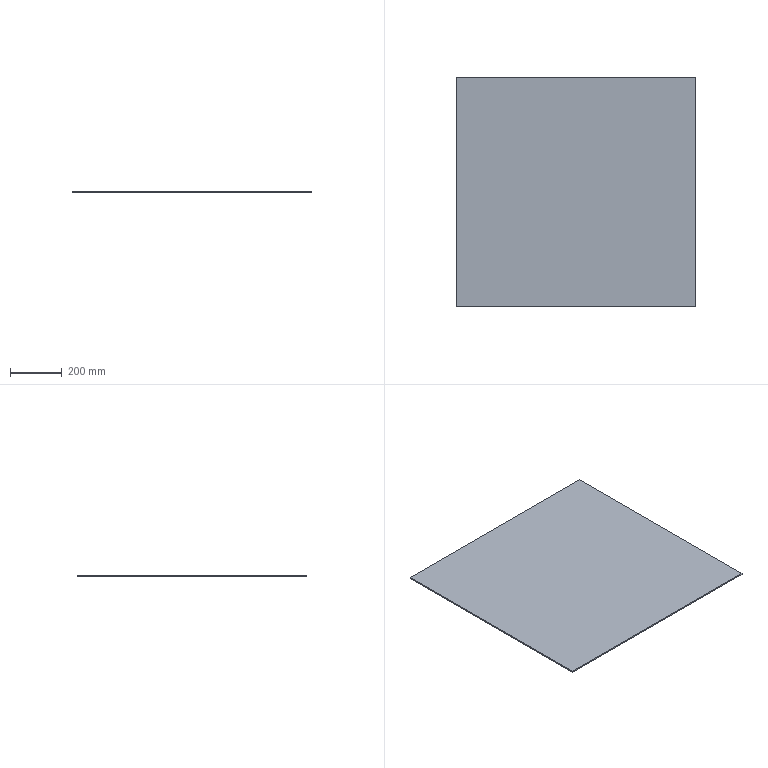Part | SolidWorks | features Extrusion 1 | 1 solid | 6 faces | box 926 x 887 x 5 mm | volume 4106810 mm3 | plane 6
STEP:
#1=CARTESIAN_POINT('',(463.,-443.5,0.));
#2=VERTEX_POINT('',#1);
#3=CARTESIAN_POINT('',(463.,443.5,0.));
#4=VERTEX_POINT('',#3);
#5=CARTESIAN_POINT('',(463.,443.5,0.));
#6=DIRECTION('',(0.,1.,0.));
#7=VECTOR('',#6,1000.);
#8=LINE('',#5,#7);
#9=EDGE_CURVE('',#2,#4,#8,.T.);
#10=ORIENTED_EDGE('',*,*,#9,.T.);
#11=CARTESIAN_POINT('',(463.,443.5,5.));
#12=VERTEX_POINT('',#11);
#13=CARTESIAN_POINT('',(463.,443.5,5.));
#14=DIRECTION('',(0.,0.,-1.));
#15=VECTOR('',#14,1000.);
#16=LINE('',#13,#15);
#17=EDGE_CURVE('',#12,#4,#16,.T.);
#18=ORIENTED_EDGE('',*,*,#17,.F.);
#19=CARTESIAN_POINT('',(463.,-443.5,5.));
#20=VERTEX_POINT('',#19);
#21=CARTESIAN_POINT('',(463.,443.5,5.));
#22=DIRECTION('',(0.,1.,0.));
#23=VECTOR('',#22,1000.);
#24=LINE('',#21,#23);
#25=EDGE_CURVE('',#20,#12,#24,.T.);
#26=ORIENTED_EDGE('',*,*,#25,.F.);
#27=CARTESIAN_POINT('',(463.,-443.5,5.));
#28=DIRECTION('',(0.,0.,-1.));
#29=VECTOR('',#28,1000.);
#30=LINE('',#27,#29);
#31=EDGE_CURVE('',#20,#2,#30,.T.);
#32=ORIENTED_EDGE('',*,*,#31,.T.);
#33=EDGE_LOOP('',(#10,#18,#26,#32));
#34=FACE_OUTER_BOUND('',#33,.T.);
#35=CARTESIAN_POINT('',(463.,443.5,5.));
#36=DIRECTION('',(-1.,0.,0.));
#37=DIRECTION('',(0.,-1.,0.));
#38=AXIS2_PLACEMENT_3D('',#35,#36,#37);
#39=PLANE('',#38);
#40=ADVANCED_FACE('',(#34),#39,.F.);
#41=CARTESIAN_POINT('',(-463.,443.5,0.));
#42=VERTEX_POINT('',#41);
#43=CARTESIAN_POINT('',(-463.,443.5,0.));
#44=DIRECTION('',(-1.,0.,0.));
#45=VECTOR('',#44,1000.);
#46=LINE('',#43,#45);
#47=EDGE_CURVE('',#4,#42,#46,.T.);
#48=ORIENTED_EDGE('',*,*,#47,.T.);
#49=CARTESIAN_POINT('',(-463.,443.5,5.));
#50=VERTEX_POINT('',#49);
#51=CARTESIAN_POINT('',(-463.,443.5,5.));
#52=DIRECTION('',(0.,0.,-1.));
#53=VECTOR('',#52,1000.);
#54=LINE('',#51,#53);
#55=EDGE_CURVE('',#50,#42,#54,.T.);
#56=ORIENTED_EDGE('',*,*,#55,.F.);
#57=CARTESIAN_POINT('',(-463.,443.5,5.));
#58=DIRECTION('',(-1.,0.,0.));
#59=VECTOR('',#58,1000.);
#60=LINE('',#57,#59);
#61=EDGE_CURVE('',#12,#50,#60,.T.);
#62=ORIENTED_EDGE('',*,*,#61,.F.);
#63=ORIENTED_EDGE('',*,*,#17,.T.);
#64=EDGE_LOOP('',(#48,#56,#62,#63));
#65=FACE_OUTER_BOUND('',#64,.T.);
#66=CARTESIAN_POINT('',(-463.,443.5,5.));
#67=DIRECTION('',(0.,-1.,0.));
#68=DIRECTION('',(0.,0.,-1.));
#69=AXIS2_PLACEMENT_3D('',#66,#67,#68);
#70=PLANE('',#69);
#71=ADVANCED_FACE('',(#65),#70,.F.);
#72=CARTESIAN_POINT('',(-463.,-443.5,0.));
#73=VERTEX_POINT('',#72);
#74=CARTESIAN_POINT('',(-463.,443.5,0.));
#75=DIRECTION('',(0.,-1.,0.));
#76=VECTOR('',#75,1000.);
#77=LINE('',#74,#76);
#78=EDGE_CURVE('',#42,#73,#77,.T.);
#79=ORIENTED_EDGE('',*,*,#78,.T.);
#80=CARTESIAN_POINT('',(-463.,-443.5,5.));
#81=VERTEX_POINT('',#80);
#82=CARTESIAN_POINT('',(-463.,-443.5,5.));
#83=DIRECTION('',(0.,0.,-1.));
#84=VECTOR('',#83,1000.);
#85=LINE('',#82,#84);
#86=EDGE_CURVE('',#81,#73,#85,.T.);
#87=ORIENTED_EDGE('',*,*,#86,.F.);
#88=CARTESIAN_POINT('',(-463.,443.5,5.));
#89=DIRECTION('',(0.,-1.,0.));
#90=VECTOR('',#89,1000.);
#91=LINE('',#88,#90);
#92=EDGE_CURVE('',#50,#81,#91,.T.);
#93=ORIENTED_EDGE('',*,*,#92,.F.);
#94=ORIENTED_EDGE('',*,*,#55,.T.);
#95=EDGE_LOOP('',(#79,#87,#93,#94));
#96=FACE_OUTER_BOUND('',#95,.T.);
#97=CARTESIAN_POINT('',(-463.,443.5,5.));
#98=DIRECTION('',(1.,0.,0.));
#99=DIRECTION('',(0.,1.,0.));
#100=AXIS2_PLACEMENT_3D('',#97,#98,#99);
#101=PLANE('',#100);
#102=ADVANCED_FACE('',(#96),#101,.F.);
#103=CARTESIAN_POINT('',(-463.,-443.5,0.));
#104=DIRECTION('',(1.,0.,0.));
#105=VECTOR('',#104,1000.);
#106=LINE('',#103,#105);
#107=EDGE_CURVE('',#73,#2,#106,.T.);
#108=ORIENTED_EDGE('',*,*,#107,.T.);
#109=ORIENTED_EDGE('',*,*,#31,.F.);
#110=CARTESIAN_POINT('',(-463.,-443.5,5.));
#111=DIRECTION('',(1.,0.,0.));
#112=VECTOR('',#111,1000.);
#113=LINE('',#110,#112);
#114=EDGE_CURVE('',#81,#20,#113,.T.);
#115=ORIENTED_EDGE('',*,*,#114,.F.);
#116=ORIENTED_EDGE('',*,*,#86,.T.);
#117=EDGE_LOOP('',(#108,#109,#115,#116));
#118=FACE_OUTER_BOUND('',#117,.T.);
#119=CARTESIAN_POINT('',(-463.,-443.5,5.));
#120=DIRECTION('',(0.,1.,0.));
#121=DIRECTION('',(0.,0.,1.));
#122=AXIS2_PLACEMENT_3D('',#119,#120,#121);
#123=PLANE('',#122);
#124=ADVANCED_FACE('',(#118),#123,.F.);
#125=ORIENTED_EDGE('',*,*,#25,.T.);
#126=ORIENTED_EDGE('',*,*,#61,.T.);
#127=ORIENTED_EDGE('',*,*,#92,.T.);
#128=ORIENTED_EDGE('',*,*,#114,.T.);
#129=EDGE_LOOP('',(#125,#126,#127,#128));
#130=FACE_OUTER_BOUND('',#129,.T.);
#131=CARTESIAN_POINT('',(0.,0.,5.));
#132=DIRECTION('',(0.,0.,1.));
#133=DIRECTION('',(1.,0.,0.));
#134=AXIS2_PLACEMENT_3D('',#131,#132,#133);
#135=PLANE('',#134);
#136=ADVANCED_FACE('',(#130),#135,.T.);
#137=ORIENTED_EDGE('',*,*,#9,.F.);
#138=ORIENTED_EDGE('',*,*,#107,.F.);
#139=ORIENTED_EDGE('',*,*,#78,.F.);
#140=ORIENTED_EDGE('',*,*,#47,.F.);
#141=EDGE_LOOP('',(#137,#138,#139,#140));
#142=FACE_OUTER_BOUND('',#141,.T.);
#143=CARTESIAN_POINT('',(0.,0.,0.));
#144=DIRECTION('',(0.,0.,1.));
#145=DIRECTION('',(1.,0.,0.));
#146=AXIS2_PLACEMENT_3D('',#143,#144,#145);
#147=PLANE('',#146);
#148=ADVANCED_FACE('',(#142),#147,.F.);
#149=CLOSED_SHELL('',(#40,#71,#102,#124,#136,#148));
#150=MANIFOLD_SOLID_BREP('',#149);
#151=CARTESIAN_POINT('',(0.,0.,0.));
#152=DIRECTION('',(0.,0.,1.));
#153=DIRECTION('',(1.,0.,0.));
#154=AXIS2_PLACEMENT_3D('',#151,#152,#153);
#155=(LENGTH_UNIT()NAMED_UNIT(*)SI_UNIT(.MILLI.,.METRE.));
#156=UNCERTAINTY_MEASURE_WITH_UNIT(LENGTH_MEASURE(0.00001),#155,'','');
#157=(NAMED_UNIT(*)PLANE_ANGLE_UNIT()SI_UNIT($,.RADIAN.));
#158=(NAMED_UNIT(*)SI_UNIT($,.STERADIAN.)SOLID_ANGLE_UNIT());
#159=(GEOMETRIC_REPRESENTATION_CONTEXT(3)GLOBAL_UNCERTAINTY_ASSIGNED_CONTEXT((#156))GLOBAL_UNIT_ASSIGNED_CONTEXT((#155,#157,#158))REPRESENTATION_CONTEXT('',''));
#160=ADVANCED_BREP_SHAPE_REPRESENTATION('',(#150,#154),#159);